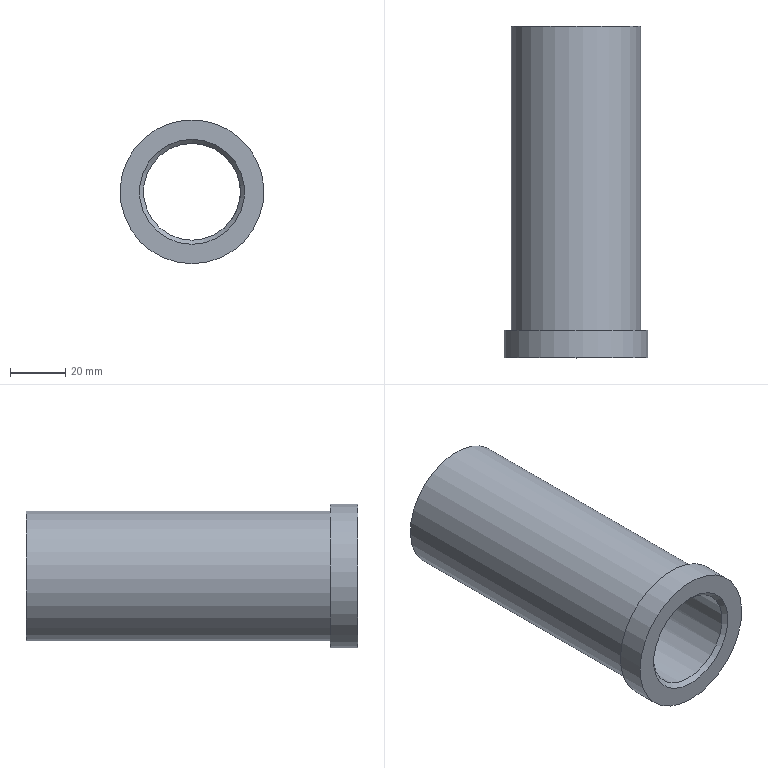Part | STEP file | GUIDE3_id238_x_t | 1 solid | 8 faces | box 52 x 120 x 52 mm | volume 96373 mm3 | cylinder 3 | plane 3 | cone 2 | commonest cylinder face diameters 35 x1 47 x1 52 x1
STEP:
#1=CARTESIAN_POINT('',(-162.,-119.,-252.5));
#2=VERTEX_POINT('',#1);
#3=CARTESIAN_POINT('',(-162.,-119.,-235.));
#4=DIRECTION('',(0.,1.,0.));
#5=DIRECTION('',(0.,0.,-1.));
#6=AXIS2_PLACEMENT_3D('',#3,#4,#5);
#7=CIRCLE('',#6,17.5);
#8=EDGE_CURVE('',#2,#2,#7,.T.);
#9=ORIENTED_EDGE('',*,*,#8,.T.);
#10=EDGE_LOOP('',(#9));
#11=FACE_BOUND('',#10,.T.);
#12=CARTESIAN_POINT('',(-162.,-120.5,-254.));
#13=VERTEX_POINT('',#12);
#14=CARTESIAN_POINT('',(-162.,-120.5,-235.));
#15=DIRECTION('',(0.,1.,0.));
#16=DIRECTION('',(0.,0.,-1.));
#17=AXIS2_PLACEMENT_3D('',#14,#15,#16);
#18=CIRCLE('',#17,19.);
#19=EDGE_CURVE('',#13,#13,#18,.T.);
#20=ORIENTED_EDGE('',*,*,#19,.F.);
#21=EDGE_LOOP('',(#20));
#22=FACE_BOUND('',#21,.T.);
#23=CARTESIAN_POINT('',(-162.,-120.5,-235.));
#24=DIRECTION('',(0.,-1.,0.));
#25=DIRECTION('',(0.,0.,-1.));
#26=AXIS2_PLACEMENT_3D('',#23,#24,#25);
#27=CONICAL_SURFACE('',#26,19.,45.);
#28=ADVANCED_FACE('',(#11,#22),#27,.F.);
#29=CARTESIAN_POINT('',(-144.5,-2.,-235.));
#30=VERTEX_POINT('',#29);
#31=CARTESIAN_POINT('',(-162.,-2.,-235.));
#32=DIRECTION('',(0.,1.,0.));
#33=DIRECTION('',(1.,0.,0.));
#34=AXIS2_PLACEMENT_3D('',#31,#32,#33);
#35=CIRCLE('',#34,17.5);
#36=EDGE_CURVE('',#30,#30,#35,.T.);
#37=ORIENTED_EDGE('',*,*,#36,.T.);
#38=EDGE_LOOP('',(#37));
#39=FACE_BOUND('',#38,.T.);
#40=ORIENTED_EDGE('',*,*,#8,.F.);
#41=EDGE_LOOP('',(#40));
#42=FACE_BOUND('',#41,.T.);
#43=CARTESIAN_POINT('',(-162.,-126.5,-235.));
#44=DIRECTION('',(0.,-1.,0.));
#45=DIRECTION('',(0.,0.,-1.));
#46=AXIS2_PLACEMENT_3D('',#43,#44,#45);
#47=CYLINDRICAL_SURFACE('',#46,17.5);
#48=ADVANCED_FACE('',(#39,#42),#47,.F.);
#49=ORIENTED_EDGE('',*,*,#19,.T.);
#50=EDGE_LOOP('',(#49));
#51=FACE_BOUND('',#50,.T.);
#52=CARTESIAN_POINT('',(-162.,-120.5,-261.));
#53=VERTEX_POINT('',#52);
#54=CARTESIAN_POINT('',(-162.,-120.5,-235.));
#55=DIRECTION('',(0.,1.,0.));
#56=DIRECTION('',(0.,0.,-1.));
#57=AXIS2_PLACEMENT_3D('',#54,#55,#56);
#58=CIRCLE('',#57,26.);
#59=EDGE_CURVE('',#53,#53,#58,.T.);
#60=ORIENTED_EDGE('',*,*,#59,.F.);
#61=EDGE_LOOP('',(#60));
#62=FACE_BOUND('',#61,.T.);
#63=CARTESIAN_POINT('',(-162.,-120.5,-235.));
#64=DIRECTION('',(0.,-1.,0.));
#65=DIRECTION('',(0.,0.,-1.));
#66=AXIS2_PLACEMENT_3D('',#63,#64,#65);
#67=PLANE('',#66);
#68=ADVANCED_FACE('',(#51,#62),#67,.T.);
#69=CARTESIAN_POINT('',(-162.,-0.5,-216.));
#70=VERTEX_POINT('',#69);
#71=CARTESIAN_POINT('',(-162.,-0.5,-235.));
#72=DIRECTION('',(0.,1.,0.));
#73=DIRECTION('',(0.,0.,1.));
#74=AXIS2_PLACEMENT_3D('',#71,#72,#73);
#75=CIRCLE('',#74,19.);
#76=EDGE_CURVE('',#70,#70,#75,.T.);
#77=ORIENTED_EDGE('',*,*,#76,.T.);
#78=EDGE_LOOP('',(#77));
#79=FACE_BOUND('',#78,.T.);
#80=ORIENTED_EDGE('',*,*,#36,.F.);
#81=EDGE_LOOP('',(#80));
#82=FACE_BOUND('',#81,.T.);
#83=CARTESIAN_POINT('',(-162.,-0.5,-235.));
#84=DIRECTION('',(0.,1.,0.));
#85=DIRECTION('',(0.,0.,1.));
#86=AXIS2_PLACEMENT_3D('',#83,#84,#85);
#87=CONICAL_SURFACE('',#86,19.,45.);
#88=ADVANCED_FACE('',(#79,#82),#87,.F.);
#89=CARTESIAN_POINT('',(-162.,-110.5,-261.));
#90=VERTEX_POINT('',#89);
#91=CARTESIAN_POINT('',(-162.,-110.5,-235.));
#92=DIRECTION('',(0.,-1.,0.));
#93=DIRECTION('',(0.,0.,-1.));
#94=AXIS2_PLACEMENT_3D('',#91,#92,#93);
#95=CIRCLE('',#94,26.);
#96=EDGE_CURVE('',#90,#90,#95,.T.);
#97=ORIENTED_EDGE('',*,*,#96,.T.);
#98=EDGE_LOOP('',(#97));
#99=FACE_BOUND('',#98,.T.);
#100=ORIENTED_EDGE('',*,*,#59,.T.);
#101=EDGE_LOOP('',(#100));
#102=FACE_BOUND('',#101,.T.);
#103=CARTESIAN_POINT('',(-162.,-126.5,-235.));
#104=DIRECTION('',(0.,-1.,0.));
#105=DIRECTION('',(0.,0.,-1.));
#106=AXIS2_PLACEMENT_3D('',#103,#104,#105);
#107=CYLINDRICAL_SURFACE('',#106,26.);
#108=ADVANCED_FACE('',(#99,#102),#107,.T.);
#109=ORIENTED_EDGE('',*,*,#76,.F.);
#110=EDGE_LOOP('',(#109));
#111=FACE_BOUND('',#110,.T.);
#112=CARTESIAN_POINT('',(-162.,-0.5,-258.5));
#113=VERTEX_POINT('',#112);
#114=CARTESIAN_POINT('',(-162.,-0.5,-235.));
#115=DIRECTION('',(0.,-1.,0.));
#116=DIRECTION('',(0.,0.,-1.));
#117=AXIS2_PLACEMENT_3D('',#114,#115,#116);
#118=CIRCLE('',#117,23.5);
#119=EDGE_CURVE('',#113,#113,#118,.T.);
#120=ORIENTED_EDGE('',*,*,#119,.F.);
#121=EDGE_LOOP('',(#120));
#122=FACE_BOUND('',#121,.T.);
#123=CARTESIAN_POINT('',(-162.,-0.5,-235.));
#124=DIRECTION('',(0.,-1.,0.));
#125=DIRECTION('',(0.,0.,-1.));
#126=AXIS2_PLACEMENT_3D('',#123,#124,#125);
#127=PLANE('',#126);
#128=ADVANCED_FACE('',(#111,#122),#127,.F.);
#129=CARTESIAN_POINT('',(-162.,-110.5,-258.5));
#130=VERTEX_POINT('',#129);
#131=CARTESIAN_POINT('',(-162.,-110.5,-235.));
#132=DIRECTION('',(0.,1.,0.));
#133=DIRECTION('',(0.,0.,-1.));
#134=AXIS2_PLACEMENT_3D('',#131,#132,#133);
#135=CIRCLE('',#134,23.5);
#136=EDGE_CURVE('',#130,#130,#135,.T.);
#137=ORIENTED_EDGE('',*,*,#136,.F.);
#138=EDGE_LOOP('',(#137));
#139=FACE_BOUND('',#138,.T.);
#140=ORIENTED_EDGE('',*,*,#96,.F.);
#141=EDGE_LOOP('',(#140));
#142=FACE_BOUND('',#141,.T.);
#143=CARTESIAN_POINT('',(-162.,-110.5,-235.));
#144=DIRECTION('',(0.,-1.,0.));
#145=DIRECTION('',(0.,0.,-1.));
#146=AXIS2_PLACEMENT_3D('',#143,#144,#145);
#147=PLANE('',#146);
#148=ADVANCED_FACE('',(#139,#142),#147,.F.);
#149=ORIENTED_EDGE('',*,*,#136,.T.);
#150=EDGE_LOOP('',(#149));
#151=FACE_BOUND('',#150,.T.);
#152=ORIENTED_EDGE('',*,*,#119,.T.);
#153=EDGE_LOOP('',(#152));
#154=FACE_BOUND('',#153,.T.);
#155=CARTESIAN_POINT('',(-162.,-126.5,-235.));
#156=DIRECTION('',(0.,-1.,0.));
#157=DIRECTION('',(0.,0.,-1.));
#158=AXIS2_PLACEMENT_3D('',#155,#156,#157);
#159=CYLINDRICAL_SURFACE('',#158,23.5);
#160=ADVANCED_FACE('',(#151,#154),#159,.T.);
#161=CLOSED_SHELL('',(#28,#48,#68,#88,#108,#128,#148,#160));
#162=MANIFOLD_SOLID_BREP('',#161);
#163=(LENGTH_UNIT()NAMED_UNIT(*)SI_UNIT(.MILLI.,.METRE.));
#164=UNCERTAINTY_MEASURE_WITH_UNIT(LENGTH_MEASURE(0.00002),#163,'','');
#165=(NAMED_UNIT(*)PLANE_ANGLE_UNIT()SI_UNIT($,.RADIAN.));
#166=PLANE_ANGLE_MEASURE_WITH_UNIT(PLANE_ANGLE_MEASURE(0.01745),#165);
#167=DIMENSIONAL_EXPONENTS(0.,0.,0.,0.,0.,0.,0.);
#168=(CONVERSION_BASED_UNIT('DEGREE',#166)NAMED_UNIT(#167)PLANE_ANGLE_UNIT());
#169=(NAMED_UNIT(*)SI_UNIT($,.STERADIAN.)SOLID_ANGLE_UNIT());
#170=(GEOMETRIC_REPRESENTATION_CONTEXT(3)GLOBAL_UNCERTAINTY_ASSIGNED_CONTEXT((#164))GLOBAL_UNIT_ASSIGNED_CONTEXT((#163,#168,#169))REPRESENTATION_CONTEXT('',''));
#171=ADVANCED_BREP_SHAPE_REPRESENTATION('',(#162),#170);